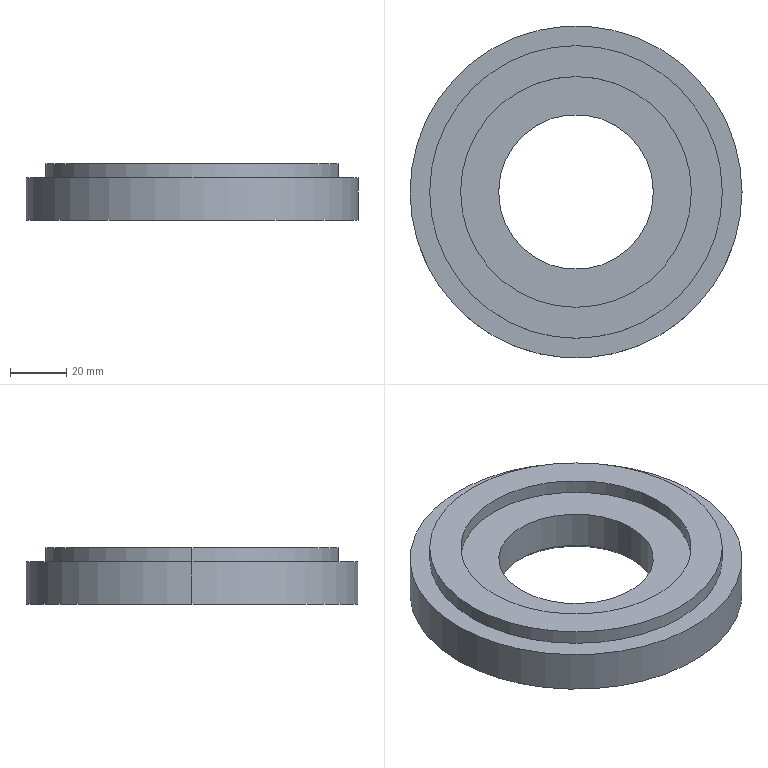Part | STEP file | Foot | 1 solid | 14 faces | box 118 x 118 x 20 mm | volume 144272 mm3 | cylinder 8 | plane 4 | cone 2 | commonest cylinder face diameters 55 x2 82 x2 104 x2 118 x2
STEP:
#1=CARTESIAN_POINT('',(0.,0.,0.));
#2=DIRECTION('',(0.,0.,1.));
#3=DIRECTION('',(1.,0.,0.));
#4=AXIS2_PLACEMENT_3D('',#1,#2,#3);
#5=CARTESIAN_POINT('',(-27.5,0.,1.5));
#6=VERTEX_POINT('',#5);
#7=CARTESIAN_POINT('',(-29.,0.,0.));
#8=VERTEX_POINT('',#7);
#9=CARTESIAN_POINT('',(-29.,0.,0.));
#10=DIRECTION('',(-0.7071,0.,-0.7071));
#11=VECTOR('',#10,1.);
#12=LINE('',#9,#11);
#13=CARTESIAN_POINT('',(0.,0.,0.));
#14=DIRECTION('',(0.,0.,-1.));
#15=DIRECTION('',(-1.,0.,0.));
#16=AXIS2_PLACEMENT_3D('',#13,#14,#15);
#17=CONICAL_SURFACE('',#16,29.,0.7854);
#18=CARTESIAN_POINT('',(6.283,0.));
#19=DIRECTION('',(0.,1.));
#20=VECTOR('',#19,1.);
#21=LINE('',#18,#20);
#22=(GEOMETRIC_REPRESENTATION_CONTEXT(2)PARAMETRIC_REPRESENTATION_CONTEXT()REPRESENTATION_CONTEXT('',''));
#23=DEFINITIONAL_REPRESENTATION('',(#21),#22);
#24=PCURVE('',#17,#23);
#25=CARTESIAN_POINT('',(0.,0.,0.));
#26=DIRECTION('',(0.,0.,-1.));
#27=DIRECTION('',(-1.,0.,0.));
#28=AXIS2_PLACEMENT_3D('',#25,#26,#27);
#29=CONICAL_SURFACE('',#28,29.,0.7854);
#30=CARTESIAN_POINT('',(0.,0.));
#31=DIRECTION('',(0.,1.));
#32=VECTOR('',#31,1.);
#33=LINE('',#30,#32);
#34=(GEOMETRIC_REPRESENTATION_CONTEXT(2)PARAMETRIC_REPRESENTATION_CONTEXT()REPRESENTATION_CONTEXT('',''));
#35=DEFINITIONAL_REPRESENTATION('',(#33),#34);
#36=PCURVE('',#29,#35);
#37=SURFACE_CURVE('',#12,(#24,#36),.PCURVE_S1.);
#38=EDGE_CURVE('',#6,#8,#37,.T.);
#39=ORIENTED_EDGE('',*,*,#38,.T.);
#40=CARTESIAN_POINT('',(29.,0.,0.));
#41=VERTEX_POINT('',#40);
#42=CARTESIAN_POINT('',(0.,0.,0.));
#43=DIRECTION('',(0.,0.,1.));
#44=DIRECTION('',(1.,0.,0.));
#45=AXIS2_PLACEMENT_3D('',#42,#43,#44);
#46=CIRCLE('',#45,29.);
#47=CARTESIAN_POINT('',(9.425,0.));
#48=DIRECTION('',(-1.,0.));
#49=VECTOR('',#48,1.);
#50=LINE('',#47,#49);
#51=(GEOMETRIC_REPRESENTATION_CONTEXT(2)PARAMETRIC_REPRESENTATION_CONTEXT()REPRESENTATION_CONTEXT('',''));
#52=DEFINITIONAL_REPRESENTATION('',(#50),#51);
#53=PCURVE('',#17,#52);
#54=CARTESIAN_POINT('',(0.,0.,0.));
#55=DIRECTION('',(0.,0.,1.));
#56=DIRECTION('',(1.,0.,0.));
#57=AXIS2_PLACEMENT_3D('',#54,#55,#56);
#58=PLANE('',#57);
#59=CARTESIAN_POINT('',(0.,0.));
#60=DIRECTION('',(1.,0.));
#61=AXIS2_PLACEMENT_2D('',#59,#60);
#62=CIRCLE('',#61,29.);
#63=(GEOMETRIC_REPRESENTATION_CONTEXT(2)PARAMETRIC_REPRESENTATION_CONTEXT()REPRESENTATION_CONTEXT('',''));
#64=DEFINITIONAL_REPRESENTATION('',(#62),#63);
#65=PCURVE('',#58,#64);
#66=SURFACE_CURVE('',#46,(#53,#65),.PCURVE_S1.);
#67=EDGE_CURVE('',#8,#41,#66,.T.);
#68=ORIENTED_EDGE('',*,*,#67,.T.);
#69=CARTESIAN_POINT('',(27.5,0.,1.5));
#70=VERTEX_POINT('',#69);
#71=CARTESIAN_POINT('',(29.,0.,0.));
#72=DIRECTION('',(0.7071,0.,-0.7071));
#73=VECTOR('',#72,1.);
#74=LINE('',#71,#73);
#75=CARTESIAN_POINT('',(3.142,0.));
#76=DIRECTION('',(0.,1.));
#77=VECTOR('',#76,1.);
#78=LINE('',#75,#77);
#79=(GEOMETRIC_REPRESENTATION_CONTEXT(2)PARAMETRIC_REPRESENTATION_CONTEXT()REPRESENTATION_CONTEXT('',''));
#80=DEFINITIONAL_REPRESENTATION('',(#78),#79);
#81=PCURVE('',#17,#80);
#82=CARTESIAN_POINT('',(3.142,0.));
#83=DIRECTION('',(0.,1.));
#84=VECTOR('',#83,1.);
#85=LINE('',#82,#84);
#86=(GEOMETRIC_REPRESENTATION_CONTEXT(2)PARAMETRIC_REPRESENTATION_CONTEXT()REPRESENTATION_CONTEXT('',''));
#87=DEFINITIONAL_REPRESENTATION('',(#85),#86);
#88=PCURVE('',#29,#87);
#89=SURFACE_CURVE('',#74,(#81,#88),.PCURVE_S1.);
#90=EDGE_CURVE('',#70,#41,#89,.T.);
#91=ORIENTED_EDGE('',*,*,#90,.F.);
#92=CARTESIAN_POINT('',(0.,0.,1.5));
#93=DIRECTION('',(0.,0.,-1.));
#94=DIRECTION('',(1.,0.,0.));
#95=AXIS2_PLACEMENT_3D('',#92,#93,#94);
#96=CIRCLE('',#95,27.5);
#97=CARTESIAN_POINT('',(3.142,-1.5));
#98=DIRECTION('',(1.,0.));
#99=VECTOR('',#98,1.);
#100=LINE('',#97,#99);
#101=(GEOMETRIC_REPRESENTATION_CONTEXT(2)PARAMETRIC_REPRESENTATION_CONTEXT()REPRESENTATION_CONTEXT('',''));
#102=DEFINITIONAL_REPRESENTATION('',(#100),#101);
#103=PCURVE('',#17,#102);
#104=CARTESIAN_POINT('',(0.,0.,15.));
#105=DIRECTION('',(0.,0.,-1.));
#106=DIRECTION('',(-1.,0.,0.));
#107=AXIS2_PLACEMENT_3D('',#104,#105,#106);
#108=CYLINDRICAL_SURFACE('',#107,27.5);
#109=CARTESIAN_POINT('',(3.142,13.5));
#110=DIRECTION('',(1.,0.));
#111=VECTOR('',#110,1.);
#112=LINE('',#109,#111);
#113=(GEOMETRIC_REPRESENTATION_CONTEXT(2)PARAMETRIC_REPRESENTATION_CONTEXT()REPRESENTATION_CONTEXT('',''));
#114=DEFINITIONAL_REPRESENTATION('',(#112),#113);
#115=PCURVE('',#108,#114);
#116=SURFACE_CURVE('',#96,(#103,#115),.PCURVE_S1.);
#117=EDGE_CURVE('',#70,#6,#116,.T.);
#118=ORIENTED_EDGE('',*,*,#117,.T.);
#119=EDGE_LOOP('',(#39,#68,#91,#118));
#120=FACE_BOUND('',#119,.F.);
#121=ADVANCED_FACE('',(#120),#17,.F.);
#122=CARTESIAN_POINT('',(-41.,0.,20.));
#123=VERTEX_POINT('',#122);
#124=CARTESIAN_POINT('',(-41.,0.,15.));
#125=VERTEX_POINT('',#124);
#126=CARTESIAN_POINT('',(-41.,0.,20.));
#127=DIRECTION('',(0.,0.,-1.));
#128=VECTOR('',#127,1.);
#129=LINE('',#126,#128);
#130=CARTESIAN_POINT('',(0.,0.,20.));
#131=DIRECTION('',(0.,0.,-1.));
#132=DIRECTION('',(-1.,0.,0.));
#133=AXIS2_PLACEMENT_3D('',#130,#131,#132);
#134=CYLINDRICAL_SURFACE('',#133,41.);
#135=CARTESIAN_POINT('',(6.283,0.));
#136=DIRECTION('',(0.,1.));
#137=VECTOR('',#136,1.);
#138=LINE('',#135,#137);
#139=(GEOMETRIC_REPRESENTATION_CONTEXT(2)PARAMETRIC_REPRESENTATION_CONTEXT()REPRESENTATION_CONTEXT('',''));
#140=DEFINITIONAL_REPRESENTATION('',(#138),#139);
#141=PCURVE('',#134,#140);
#142=CARTESIAN_POINT('',(0.,0.,20.));
#143=DIRECTION('',(0.,0.,-1.));
#144=DIRECTION('',(-1.,0.,0.));
#145=AXIS2_PLACEMENT_3D('',#142,#143,#144);
#146=CYLINDRICAL_SURFACE('',#145,41.);
#147=CARTESIAN_POINT('',(0.,0.));
#148=DIRECTION('',(0.,1.));
#149=VECTOR('',#148,1.);
#150=LINE('',#147,#149);
#151=(GEOMETRIC_REPRESENTATION_CONTEXT(2)PARAMETRIC_REPRESENTATION_CONTEXT()REPRESENTATION_CONTEXT('',''));
#152=DEFINITIONAL_REPRESENTATION('',(#150),#151);
#153=PCURVE('',#146,#152);
#154=SURFACE_CURVE('',#129,(#141,#153),.PCURVE_S1.);
#155=EDGE_CURVE('',#123,#125,#154,.T.);
#156=ORIENTED_EDGE('',*,*,#155,.T.);
#157=CARTESIAN_POINT('',(41.,0.,15.));
#158=VERTEX_POINT('',#157);
#159=CARTESIAN_POINT('',(0.,0.,15.));
#160=DIRECTION('',(0.,0.,-1.));
#161=DIRECTION('',(1.,0.,0.));
#162=AXIS2_PLACEMENT_3D('',#159,#160,#161);
#163=CIRCLE('',#162,41.);
#164=CARTESIAN_POINT('',(3.142,5.));
#165=DIRECTION('',(1.,0.));
#166=VECTOR('',#165,1.);
#167=LINE('',#164,#166);
#168=(GEOMETRIC_REPRESENTATION_CONTEXT(2)PARAMETRIC_REPRESENTATION_CONTEXT()REPRESENTATION_CONTEXT('',''));
#169=DEFINITIONAL_REPRESENTATION('',(#167),#168);
#170=PCURVE('',#134,#169);
#171=CARTESIAN_POINT('',(0.,0.,15.));
#172=DIRECTION('',(0.,0.,1.));
#173=DIRECTION('',(1.,0.,0.));
#174=AXIS2_PLACEMENT_3D('',#171,#172,#173);
#175=PLANE('',#174);
#176=CARTESIAN_POINT('',(41.,0.));
#177=CARTESIAN_POINT('',(41.,-71.014));
#178=CARTESIAN_POINT('',(-20.5,-35.507));
#179=CARTESIAN_POINT('',(-82.,0.));
#180=CARTESIAN_POINT('',(-20.5,35.507));
#181=CARTESIAN_POINT('',(41.,71.014));
#182=CARTESIAN_POINT('',(41.,0.));
#183=(BOUNDED_CURVE()B_SPLINE_CURVE(2,(#176,#177,#178,#179,#180,#181,#182),.UNSPECIFIED.,.T.,.F.)B_SPLINE_CURVE_WITH_KNOTS((1,2,2,2,2,1),(-2.094,0.,2.094,4.189,6.283,8.378),.UNSPECIFIED.)CURVE()GEOMETRIC_REPRESENTATION_ITEM()RATIONAL_B_SPLINE_CURVE((1.,0.5,1.,0.5,1.,0.5,1.))REPRESENTATION_ITEM(''));
#184=(GEOMETRIC_REPRESENTATION_CONTEXT(2)PARAMETRIC_REPRESENTATION_CONTEXT()REPRESENTATION_CONTEXT('',''));
#185=DEFINITIONAL_REPRESENTATION('',(#183),#184);
#186=PCURVE('',#175,#185);
#187=SURFACE_CURVE('',#163,(#170,#186),.PCURVE_S1.);
#188=EDGE_CURVE('',#158,#125,#187,.T.);
#189=ORIENTED_EDGE('',*,*,#188,.F.);
#190=CARTESIAN_POINT('',(41.,0.,20.));
#191=VERTEX_POINT('',#190);
#192=CARTESIAN_POINT('',(41.,0.,20.));
#193=DIRECTION('',(0.,0.,-1.));
#194=VECTOR('',#193,1.);
#195=LINE('',#192,#194);
#196=CARTESIAN_POINT('',(3.142,0.));
#197=DIRECTION('',(0.,1.));
#198=VECTOR('',#197,1.);
#199=LINE('',#196,#198);
#200=(GEOMETRIC_REPRESENTATION_CONTEXT(2)PARAMETRIC_REPRESENTATION_CONTEXT()REPRESENTATION_CONTEXT('',''));
#201=DEFINITIONAL_REPRESENTATION('',(#199),#200);
#202=PCURVE('',#134,#201);
#203=CARTESIAN_POINT('',(3.142,0.));
#204=DIRECTION('',(0.,1.));
#205=VECTOR('',#204,1.);
#206=LINE('',#203,#205);
#207=(GEOMETRIC_REPRESENTATION_CONTEXT(2)PARAMETRIC_REPRESENTATION_CONTEXT()REPRESENTATION_CONTEXT('',''));
#208=DEFINITIONAL_REPRESENTATION('',(#206),#207);
#209=PCURVE('',#146,#208);
#210=SURFACE_CURVE('',#195,(#202,#209),.PCURVE_S1.);
#211=EDGE_CURVE('',#191,#158,#210,.T.);
#212=ORIENTED_EDGE('',*,*,#211,.F.);
#213=CARTESIAN_POINT('',(0.,0.,20.));
#214=DIRECTION('',(0.,0.,1.));
#215=DIRECTION('',(1.,0.,0.));
#216=AXIS2_PLACEMENT_3D('',#213,#214,#215);
#217=CIRCLE('',#216,41.);
#218=CARTESIAN_POINT('',(9.425,0.));
#219=DIRECTION('',(-1.,0.));
#220=VECTOR('',#219,1.);
#221=LINE('',#218,#220);
#222=(GEOMETRIC_REPRESENTATION_CONTEXT(2)PARAMETRIC_REPRESENTATION_CONTEXT()REPRESENTATION_CONTEXT('',''));
#223=DEFINITIONAL_REPRESENTATION('',(#221),#222);
#224=PCURVE('',#134,#223);
#225=CARTESIAN_POINT('',(0.,0.,20.));
#226=DIRECTION('',(0.,0.,1.));
#227=DIRECTION('',(1.,0.,0.));
#228=AXIS2_PLACEMENT_3D('',#225,#226,#227);
#229=PLANE('',#228);
#230=CARTESIAN_POINT('',(0.,0.));
#231=DIRECTION('',(1.,0.));
#232=AXIS2_PLACEMENT_2D('',#230,#231);
#233=CIRCLE('',#232,41.);
#234=(GEOMETRIC_REPRESENTATION_CONTEXT(2)PARAMETRIC_REPRESENTATION_CONTEXT()REPRESENTATION_CONTEXT('',''));
#235=DEFINITIONAL_REPRESENTATION('',(#233),#234);
#236=PCURVE('',#229,#235);
#237=SURFACE_CURVE('',#217,(#224,#236),.PCURVE_S1.);
#238=EDGE_CURVE('',#123,#191,#237,.T.);
#239=ORIENTED_EDGE('',*,*,#238,.F.);
#240=EDGE_LOOP('',(#156,#189,#212,#239));
#241=FACE_BOUND('',#240,.F.);
#242=ADVANCED_FACE('',(#241),#134,.F.);
#243=CARTESIAN_POINT('',(52.,0.,20.));
#244=VERTEX_POINT('',#243);
#245=CARTESIAN_POINT('',(-52.,0.,20.));
#246=VERTEX_POINT('',#245);
#247=CARTESIAN_POINT('',(0.,0.,20.));
#248=DIRECTION('',(0.,0.,1.));
#249=DIRECTION('',(1.,0.,0.));
#250=AXIS2_PLACEMENT_3D('',#247,#248,#249);
#251=CIRCLE('',#250,52.);
#252=CARTESIAN_POINT('',(0.,0.,20.));
#253=DIRECTION('',(0.,0.,-1.));
#254=DIRECTION('',(-1.,0.,0.));
#255=AXIS2_PLACEMENT_3D('',#252,#253,#254);
#256=CYLINDRICAL_SURFACE('',#255,52.);
#257=CARTESIAN_POINT('',(3.142,0.));
#258=DIRECTION('',(-1.,0.));
#259=VECTOR('',#258,1.);
#260=LINE('',#257,#259);
#261=(GEOMETRIC_REPRESENTATION_CONTEXT(2)PARAMETRIC_REPRESENTATION_CONTEXT()REPRESENTATION_CONTEXT('',''));
#262=DEFINITIONAL_REPRESENTATION('',(#260),#261);
#263=PCURVE('',#256,#262);
#264=CARTESIAN_POINT('',(0.,0.));
#265=DIRECTION('',(1.,0.));
#266=AXIS2_PLACEMENT_2D('',#264,#265);
#267=CIRCLE('',#266,52.);
#268=(GEOMETRIC_REPRESENTATION_CONTEXT(2)PARAMETRIC_REPRESENTATION_CONTEXT()REPRESENTATION_CONTEXT('',''));
#269=DEFINITIONAL_REPRESENTATION('',(#267),#268);
#270=PCURVE('',#229,#269);
#271=SURFACE_CURVE('',#251,(#263,#270),.PCURVE_S1.);
#272=EDGE_CURVE('',#244,#246,#271,.T.);
#273=ORIENTED_EDGE('',*,*,#272,.F.);
#274=CARTESIAN_POINT('',(52.,0.,15.));
#275=VERTEX_POINT('',#274);
#276=CARTESIAN_POINT('',(52.,0.,20.));
#277=DIRECTION('',(0.,0.,-1.));
#278=VECTOR('',#277,1.);
#279=LINE('',#276,#278);
#280=CARTESIAN_POINT('',(3.142,0.));
#281=DIRECTION('',(0.,1.));
#282=VECTOR('',#281,1.);
#283=LINE('',#280,#282);
#284=(GEOMETRIC_REPRESENTATION_CONTEXT(2)PARAMETRIC_REPRESENTATION_CONTEXT()REPRESENTATION_CONTEXT('',''));
#285=DEFINITIONAL_REPRESENTATION('',(#283),#284);
#286=PCURVE('',#256,#285);
#287=CARTESIAN_POINT('',(0.,0.,20.));
#288=DIRECTION('',(0.,0.,-1.));
#289=DIRECTION('',(-1.,0.,0.));
#290=AXIS2_PLACEMENT_3D('',#287,#288,#289);
#291=CYLINDRICAL_SURFACE('',#290,52.);
#292=CARTESIAN_POINT('',(3.142,0.));
#293=DIRECTION('',(0.,1.));
#294=VECTOR('',#293,1.);
#295=LINE('',#292,#294);
#296=(GEOMETRIC_REPRESENTATION_CONTEXT(2)PARAMETRIC_REPRESENTATION_CONTEXT()REPRESENTATION_CONTEXT('',''));
#297=DEFINITIONAL_REPRESENTATION('',(#295),#296);
#298=PCURVE('',#291,#297);
#299=SURFACE_CURVE('',#279,(#286,#298),.PCURVE_S1.);
#300=EDGE_CURVE('',#244,#275,#299,.T.);
#301=ORIENTED_EDGE('',*,*,#300,.T.);
#302=CARTESIAN_POINT('',(-52.,0.,15.));
#303=VERTEX_POINT('',#302);
#304=CARTESIAN_POINT('',(0.,0.,15.));
#305=DIRECTION('',(0.,0.,1.));
#306=DIRECTION('',(1.,0.,0.));
#307=AXIS2_PLACEMENT_3D('',#304,#305,#306);
#308=CIRCLE('',#307,52.);
#309=CARTESIAN_POINT('',(3.142,5.));
#310=DIRECTION('',(-1.,0.));
#311=VECTOR('',#310,1.);
#312=LINE('',#309,#311);
#313=(GEOMETRIC_REPRESENTATION_CONTEXT(2)PARAMETRIC_REPRESENTATION_CONTEXT()REPRESENTATION_CONTEXT('',''));
#314=DEFINITIONAL_REPRESENTATION('',(#312),#313);
#315=PCURVE('',#256,#314);
#316=CARTESIAN_POINT('',(0.,0.,15.));
#317=DIRECTION('',(0.,0.,1.));
#318=DIRECTION('',(1.,0.,0.));
#319=AXIS2_PLACEMENT_3D('',#316,#317,#318);
#320=PLANE('',#319);
#321=CARTESIAN_POINT('',(0.,0.));
#322=DIRECTION('',(1.,0.));
#323=AXIS2_PLACEMENT_2D('',#321,#322);
#324=CIRCLE('',#323,52.);
#325=(GEOMETRIC_REPRESENTATION_CONTEXT(2)PARAMETRIC_REPRESENTATION_CONTEXT()REPRESENTATION_CONTEXT('',''));
#326=DEFINITIONAL_REPRESENTATION('',(#324),#325);
#327=PCURVE('',#320,#326);
#328=SURFACE_CURVE('',#308,(#315,#327),.PCURVE_S1.);
#329=EDGE_CURVE('',#275,#303,#328,.T.);
#330=ORIENTED_EDGE('',*,*,#329,.T.);
#331=CARTESIAN_POINT('',(-52.,0.,20.));
#332=DIRECTION('',(0.,0.,-1.));
#333=VECTOR('',#332,1.);
#334=LINE('',#331,#333);
#335=CARTESIAN_POINT('',(0.,0.));
#336=DIRECTION('',(0.,1.));
#337=VECTOR('',#336,1.);
#338=LINE('',#335,#337);
#339=(GEOMETRIC_REPRESENTATION_CONTEXT(2)PARAMETRIC_REPRESENTATION_CONTEXT()REPRESENTATION_CONTEXT('',''));
#340=DEFINITIONAL_REPRESENTATION('',(#338),#339);
#341=PCURVE('',#256,#340);
#342=CARTESIAN_POINT('',(6.283,0.));
#343=DIRECTION('',(0.,1.));
#344=VECTOR('',#343,1.);
#345=LINE('',#342,#344);
#346=(GEOMETRIC_REPRESENTATION_CONTEXT(2)PARAMETRIC_REPRESENTATION_CONTEXT()REPRESENTATION_CONTEXT('',''));
#347=DEFINITIONAL_REPRESENTATION('',(#345),#346);
#348=PCURVE('',#291,#347);
#349=SURFACE_CURVE('',#334,(#341,#348),.PCURVE_S1.);
#350=EDGE_CURVE('',#246,#303,#349,.T.);
#351=ORIENTED_EDGE('',*,*,#350,.F.);
#352=EDGE_LOOP('',(#273,#301,#330,#351));
#353=FACE_BOUND('',#352,.T.);
#354=ADVANCED_FACE('',(#353),#256,.T.);
#355=CARTESIAN_POINT('',(-27.5,0.,15.));
#356=VERTEX_POINT('',#355);
#357=CARTESIAN_POINT('',(-27.5,0.,15.));
#358=DIRECTION('',(0.,0.,-1.));
#359=VECTOR('',#358,1.);
#360=LINE('',#357,#359);
#361=CARTESIAN_POINT('',(6.283,0.));
#362=DIRECTION('',(0.,1.));
#363=VECTOR('',#362,1.);
#364=LINE('',#361,#363);
#365=(GEOMETRIC_REPRESENTATION_CONTEXT(2)PARAMETRIC_REPRESENTATION_CONTEXT()REPRESENTATION_CONTEXT('',''));
#366=DEFINITIONAL_REPRESENTATION('',(#364),#365);
#367=PCURVE('',#108,#366);
#368=CARTESIAN_POINT('',(0.,0.,15.));
#369=DIRECTION('',(0.,0.,-1.));
#370=DIRECTION('',(-1.,0.,0.));
#371=AXIS2_PLACEMENT_3D('',#368,#369,#370);
#372=CYLINDRICAL_SURFACE('',#371,27.5);
#373=CARTESIAN_POINT('',(0.,0.));
#374=DIRECTION('',(0.,1.));
#375=VECTOR('',#374,1.);
#376=LINE('',#373,#375);
#377=(GEOMETRIC_REPRESENTATION_CONTEXT(2)PARAMETRIC_REPRESENTATION_CONTEXT()REPRESENTATION_CONTEXT('',''));
#378=DEFINITIONAL_REPRESENTATION('',(#376),#377);
#379=PCURVE('',#372,#378);
#380=SURFACE_CURVE('',#360,(#367,#379),.PCURVE_S1.);
#381=EDGE_CURVE('',#356,#6,#380,.T.);
#382=ORIENTED_EDGE('',*,*,#381,.T.);
#383=ORIENTED_EDGE('',*,*,#117,.F.);
#384=CARTESIAN_POINT('',(27.5,0.,15.));
#385=VERTEX_POINT('',#384);
#386=CARTESIAN_POINT('',(27.5,0.,15.));
#387=DIRECTION('',(0.,0.,-1.));
#388=VECTOR('',#387,1.);
#389=LINE('',#386,#388);
#390=CARTESIAN_POINT('',(3.142,0.));
#391=DIRECTION('',(0.,1.));
#392=VECTOR('',#391,1.);
#393=LINE('',#390,#392);
#394=(GEOMETRIC_REPRESENTATION_CONTEXT(2)PARAMETRIC_REPRESENTATION_CONTEXT()REPRESENTATION_CONTEXT('',''));
#395=DEFINITIONAL_REPRESENTATION('',(#393),#394);
#396=PCURVE('',#108,#395);
#397=CARTESIAN_POINT('',(3.142,0.));
#398=DIRECTION('',(0.,1.));
#399=VECTOR('',#398,1.);
#400=LINE('',#397,#399);
#401=(GEOMETRIC_REPRESENTATION_CONTEXT(2)PARAMETRIC_REPRESENTATION_CONTEXT()REPRESENTATION_CONTEXT('',''));
#402=DEFINITIONAL_REPRESENTATION('',(#400),#401);
#403=PCURVE('',#372,#402);
#404=SURFACE_CURVE('',#389,(#396,#403),.PCURVE_S1.);
#405=EDGE_CURVE('',#385,#70,#404,.T.);
#406=ORIENTED_EDGE('',*,*,#405,.F.);
#407=CARTESIAN_POINT('',(0.,0.,15.));
#408=DIRECTION('',(0.,0.,1.));
#409=DIRECTION('',(1.,0.,0.));
#410=AXIS2_PLACEMENT_3D('',#407,#408,#409);
#411=CIRCLE('',#410,27.5);
#412=CARTESIAN_POINT('',(9.425,0.));
#413=DIRECTION('',(-1.,0.));
#414=VECTOR('',#413,1.);
#415=LINE('',#412,#414);
#416=(GEOMETRIC_REPRESENTATION_CONTEXT(2)PARAMETRIC_REPRESENTATION_CONTEXT()REPRESENTATION_CONTEXT('',''));
#417=DEFINITIONAL_REPRESENTATION('',(#415),#416);
#418=PCURVE('',#108,#417);
#419=CARTESIAN_POINT('',(0.,0.));
#420=DIRECTION('',(1.,0.));
#421=AXIS2_PLACEMENT_2D('',#419,#420);
#422=CIRCLE('',#421,27.5);
#423=(GEOMETRIC_REPRESENTATION_CONTEXT(2)PARAMETRIC_REPRESENTATION_CONTEXT()REPRESENTATION_CONTEXT('',''));
#424=DEFINITIONAL_REPRESENTATION('',(#422),#423);
#425=PCURVE('',#175,#424);
#426=SURFACE_CURVE('',#411,(#418,#425),.PCURVE_S1.);
#427=EDGE_CURVE('',#356,#385,#426,.T.);
#428=ORIENTED_EDGE('',*,*,#427,.F.);
#429=EDGE_LOOP('',(#382,#383,#406,#428));
#430=FACE_BOUND('',#429,.F.);
#431=ADVANCED_FACE('',(#430),#108,.F.);
#432=CARTESIAN_POINT('',(59.,0.,15.));
#433=VERTEX_POINT('',#432);
#434=CARTESIAN_POINT('',(-59.,0.,15.));
#435=VERTEX_POINT('',#434);
#436=CARTESIAN_POINT('',(0.,0.,15.));
#437=DIRECTION('',(0.,0.,1.));
#438=DIRECTION('',(1.,0.,0.));
#439=AXIS2_PLACEMENT_3D('',#436,#437,#438);
#440=CIRCLE('',#439,59.);
#441=CARTESIAN_POINT('',(0.,0.,15.));
#442=DIRECTION('',(0.,0.,-1.));
#443=DIRECTION('',(-1.,0.,0.));
#444=AXIS2_PLACEMENT_3D('',#441,#442,#443);
#445=CYLINDRICAL_SURFACE('',#444,59.);
#446=CARTESIAN_POINT('',(3.142,0.));
#447=DIRECTION('',(-1.,0.));
#448=VECTOR('',#447,1.);
#449=LINE('',#446,#448);
#450=(GEOMETRIC_REPRESENTATION_CONTEXT(2)PARAMETRIC_REPRESENTATION_CONTEXT()REPRESENTATION_CONTEXT('',''));
#451=DEFINITIONAL_REPRESENTATION('',(#449),#450);
#452=PCURVE('',#445,#451);
#453=CARTESIAN_POINT('',(0.,0.));
#454=DIRECTION('',(1.,0.));
#455=AXIS2_PLACEMENT_2D('',#453,#454);
#456=CIRCLE('',#455,59.);
#457=(GEOMETRIC_REPRESENTATION_CONTEXT(2)PARAMETRIC_REPRESENTATION_CONTEXT()REPRESENTATION_CONTEXT('',''));
#458=DEFINITIONAL_REPRESENTATION('',(#456),#457);
#459=PCURVE('',#320,#458);
#460=SURFACE_CURVE('',#440,(#452,#459),.PCURVE_S1.);
#461=EDGE_CURVE('',#433,#435,#460,.T.);
#462=ORIENTED_EDGE('',*,*,#461,.F.);
#463=CARTESIAN_POINT('',(59.,0.,0.));
#464=VERTEX_POINT('',#463);
#465=CARTESIAN_POINT('',(59.,0.,15.));
#466=DIRECTION('',(0.,0.,-1.));
#467=VECTOR('',#466,1.);
#468=LINE('',#465,#467);
#469=CARTESIAN_POINT('',(3.142,0.));
#470=DIRECTION('',(0.,1.));
#471=VECTOR('',#470,1.);
#472=LINE('',#469,#471);
#473=(GEOMETRIC_REPRESENTATION_CONTEXT(2)PARAMETRIC_REPRESENTATION_CONTEXT()REPRESENTATION_CONTEXT('',''));
#474=DEFINITIONAL_REPRESENTATION('',(#472),#473);
#475=PCURVE('',#445,#474);
#476=CARTESIAN_POINT('',(0.,0.,15.));
#477=DIRECTION('',(0.,0.,-1.));
#478=DIRECTION('',(-1.,0.,0.));
#479=AXIS2_PLACEMENT_3D('',#476,#477,#478);
#480=CYLINDRICAL_SURFACE('',#479,59.);
#481=CARTESIAN_POINT('',(3.142,0.));
#482=DIRECTION('',(0.,1.));
#483=VECTOR('',#482,1.);
#484=LINE('',#481,#483);
#485=(GEOMETRIC_REPRESENTATION_CONTEXT(2)PARAMETRIC_REPRESENTATION_CONTEXT()REPRESENTATION_CONTEXT('',''));
#486=DEFINITIONAL_REPRESENTATION('',(#484),#485);
#487=PCURVE('',#480,#486);
#488=SURFACE_CURVE('',#468,(#475,#487),.PCURVE_S1.);
#489=EDGE_CURVE('',#433,#464,#488,.T.);
#490=ORIENTED_EDGE('',*,*,#489,.T.);
#491=CARTESIAN_POINT('',(-59.,0.,0.));
#492=VERTEX_POINT('',#491);
#493=CARTESIAN_POINT('',(0.,0.,0.));
#494=DIRECTION('',(0.,0.,1.));
#495=DIRECTION('',(1.,0.,0.));
#496=AXIS2_PLACEMENT_3D('',#493,#494,#495);
#497=CIRCLE('',#496,59.);
#498=CARTESIAN_POINT('',(3.142,15.));
#499=DIRECTION('',(-1.,0.));
#500=VECTOR('',#499,1.);
#501=LINE('',#498,#500);
#502=(GEOMETRIC_REPRESENTATION_CONTEXT(2)PARAMETRIC_REPRESENTATION_CONTEXT()REPRESENTATION_CONTEXT('',''));
#503=DEFINITIONAL_REPRESENTATION('',(#501),#502);
#504=PCURVE('',#445,#503);
#505=CARTESIAN_POINT('',(0.,0.));
#506=DIRECTION('',(1.,0.));
#507=AXIS2_PLACEMENT_2D('',#505,#506);
#508=CIRCLE('',#507,59.);
#509=(GEOMETRIC_REPRESENTATION_CONTEXT(2)PARAMETRIC_REPRESENTATION_CONTEXT()REPRESENTATION_CONTEXT('',''));
#510=DEFINITIONAL_REPRESENTATION('',(#508),#509);
#511=PCURVE('',#58,#510);
#512=SURFACE_CURVE('',#497,(#504,#511),.PCURVE_S1.);
#513=EDGE_CURVE('',#464,#492,#512,.T.);
#514=ORIENTED_EDGE('',*,*,#513,.T.);
#515=CARTESIAN_POINT('',(-59.,0.,15.));
#516=DIRECTION('',(0.,0.,-1.));
#517=VECTOR('',#516,1.);
#518=LINE('',#515,#517);
#519=CARTESIAN_POINT('',(0.,0.));
#520=DIRECTION('',(0.,1.));
#521=VECTOR('',#520,1.);
#522=LINE('',#519,#521);
#523=(GEOMETRIC_REPRESENTATION_CONTEXT(2)PARAMETRIC_REPRESENTATION_CONTEXT()REPRESENTATION_CONTEXT('',''));
#524=DEFINITIONAL_REPRESENTATION('',(#522),#523);
#525=PCURVE('',#445,#524);
#526=CARTESIAN_POINT('',(6.283,0.));
#527=DIRECTION('',(0.,1.));
#528=VECTOR('',#527,1.);
#529=LINE('',#526,#528);
#530=(GEOMETRIC_REPRESENTATION_CONTEXT(2)PARAMETRIC_REPRESENTATION_CONTEXT()REPRESENTATION_CONTEXT('',''));
#531=DEFINITIONAL_REPRESENTATION('',(#529),#530);
#532=PCURVE('',#480,#531);
#533=SURFACE_CURVE('',#518,(#525,#532),.PCURVE_S1.);
#534=EDGE_CURVE('',#435,#492,#533,.T.);
#535=ORIENTED_EDGE('',*,*,#534,.F.);
#536=EDGE_LOOP('',(#462,#490,#514,#535));
#537=FACE_BOUND('',#536,.T.);
#538=ADVANCED_FACE('',(#537),#445,.T.);
#539=CARTESIAN_POINT('',(0.,0.,15.));
#540=DIRECTION('',(0.,0.,1.));
#541=DIRECTION('',(1.,0.,0.));
#542=AXIS2_PLACEMENT_3D('',#539,#540,#541);
#543=CIRCLE('',#542,59.);
#544=CARTESIAN_POINT('',(0.,0.));
#545=DIRECTION('',(1.,0.));
#546=AXIS2_PLACEMENT_2D('',#544,#545);
#547=CIRCLE('',#546,59.);
#548=(GEOMETRIC_REPRESENTATION_CONTEXT(2)PARAMETRIC_REPRESENTATION_CONTEXT()REPRESENTATION_CONTEXT('',''));
#549=DEFINITIONAL_REPRESENTATION('',(#547),#548);
#550=PCURVE('',#320,#549);
#551=CARTESIAN_POINT('',(9.425,0.));
#552=DIRECTION('',(-1.,0.));
#553=VECTOR('',#552,1.);
#554=LINE('',#551,#553);
#555=(GEOMETRIC_REPRESENTATION_CONTEXT(2)PARAMETRIC_REPRESENTATION_CONTEXT()REPRESENTATION_CONTEXT('',''));
#556=DEFINITIONAL_REPRESENTATION('',(#554),#555);
#557=PCURVE('',#480,#556);
#558=SURFACE_CURVE('',#543,(#550,#557),.PCURVE_S1.);
#559=EDGE_CURVE('',#435,#433,#558,.T.);
#560=ORIENTED_EDGE('',*,*,#559,.T.);
#561=ORIENTED_EDGE('',*,*,#461,.T.);
#562=EDGE_LOOP('',(#560,#561));
#563=FACE_BOUND('',#562,.T.);
#564=CARTESIAN_POINT('',(0.,0.,15.));
#565=DIRECTION('',(0.,0.,1.));
#566=DIRECTION('',(1.,0.,0.));
#567=AXIS2_PLACEMENT_3D('',#564,#565,#566);
#568=CIRCLE('',#567,52.);
#569=CARTESIAN_POINT('',(0.,0.));
#570=DIRECTION('',(1.,0.));
#571=AXIS2_PLACEMENT_2D('',#569,#570);
#572=CIRCLE('',#571,52.);
#573=(GEOMETRIC_REPRESENTATION_CONTEXT(2)PARAMETRIC_REPRESENTATION_CONTEXT()REPRESENTATION_CONTEXT('',''));
#574=DEFINITIONAL_REPRESENTATION('',(#572),#573);
#575=PCURVE('',#320,#574);
#576=CARTESIAN_POINT('',(9.425,5.));
#577=DIRECTION('',(-1.,0.));
#578=VECTOR('',#577,1.);
#579=LINE('',#576,#578);
#580=(GEOMETRIC_REPRESENTATION_CONTEXT(2)PARAMETRIC_REPRESENTATION_CONTEXT()REPRESENTATION_CONTEXT('',''));
#581=DEFINITIONAL_REPRESENTATION('',(#579),#580);
#582=PCURVE('',#291,#581);
#583=SURFACE_CURVE('',#568,(#575,#582),.PCURVE_S1.);
#584=EDGE_CURVE('',#303,#275,#583,.T.);
#585=ORIENTED_EDGE('',*,*,#584,.F.);
#586=ORIENTED_EDGE('',*,*,#329,.F.);
#587=EDGE_LOOP('',(#585,#586));
#588=FACE_BOUND('',#587,.T.);
#589=ADVANCED_FACE('',(#563,#588),#320,.T.);
#590=CARTESIAN_POINT('',(0.,0.,15.));
#591=DIRECTION('',(0.,0.,-1.));
#592=DIRECTION('',(1.,0.,0.));
#593=AXIS2_PLACEMENT_3D('',#590,#591,#592);
#594=CIRCLE('',#593,41.);
#595=CARTESIAN_POINT('',(41.,0.));
#596=CARTESIAN_POINT('',(41.,-71.014));
#597=CARTESIAN_POINT('',(-20.5,-35.507));
#598=CARTESIAN_POINT('',(-82.,0.));
#599=CARTESIAN_POINT('',(-20.5,35.507));
#600=CARTESIAN_POINT('',(41.,71.014));
#601=CARTESIAN_POINT('',(41.,0.));
#602=(BOUNDED_CURVE()B_SPLINE_CURVE(2,(#595,#596,#597,#598,#599,#600,#601),.UNSPECIFIED.,.T.,.F.)B_SPLINE_CURVE_WITH_KNOTS((1,2,2,2,2,1),(-2.094,0.,2.094,4.189,6.283,8.378),.UNSPECIFIED.)CURVE()GEOMETRIC_REPRESENTATION_ITEM()RATIONAL_B_SPLINE_CURVE((1.,0.5,1.,0.5,1.,0.5,1.))REPRESENTATION_ITEM(''));
#603=(GEOMETRIC_REPRESENTATION_CONTEXT(2)PARAMETRIC_REPRESENTATION_CONTEXT()REPRESENTATION_CONTEXT('',''));
#604=DEFINITIONAL_REPRESENTATION('',(#602),#603);
#605=PCURVE('',#175,#604);
#606=CARTESIAN_POINT('',(-3.142,5.));
#607=DIRECTION('',(1.,0.));
#608=VECTOR('',#607,1.);
#609=LINE('',#606,#608);
#610=(GEOMETRIC_REPRESENTATION_CONTEXT(2)PARAMETRIC_REPRESENTATION_CONTEXT()REPRESENTATION_CONTEXT('',''));
#611=DEFINITIONAL_REPRESENTATION('',(#609),#610);
#612=PCURVE('',#146,#611);
#613=SURFACE_CURVE('',#594,(#605,#612),.PCURVE_S1.);
#614=EDGE_CURVE('',#125,#158,#613,.T.);
#615=ORIENTED_EDGE('',*,*,#614,.F.);
#616=ORIENTED_EDGE('',*,*,#188,.F.);
#617=EDGE_LOOP('',(#615,#616));
#618=FACE_BOUND('',#617,.T.);
#619=ORIENTED_EDGE('',*,*,#427,.F.);
#620=CARTESIAN_POINT('',(0.,0.,15.));
#621=DIRECTION('',(0.,0.,1.));
#622=DIRECTION('',(1.,0.,0.));
#623=AXIS2_PLACEMENT_3D('',#620,#621,#622);
#624=CIRCLE('',#623,27.5);
#625=CARTESIAN_POINT('',(0.,0.));
#626=DIRECTION('',(1.,0.));
#627=AXIS2_PLACEMENT_2D('',#625,#626);
#628=CIRCLE('',#627,27.5);
#629=(GEOMETRIC_REPRESENTATION_CONTEXT(2)PARAMETRIC_REPRESENTATION_CONTEXT()REPRESENTATION_CONTEXT('',''));
#630=DEFINITIONAL_REPRESENTATION('',(#628),#629);
#631=PCURVE('',#175,#630);
#632=CARTESIAN_POINT('',(3.142,0.));
#633=DIRECTION('',(-1.,0.));
#634=VECTOR('',#633,1.);
#635=LINE('',#632,#634);
#636=(GEOMETRIC_REPRESENTATION_CONTEXT(2)PARAMETRIC_REPRESENTATION_CONTEXT()REPRESENTATION_CONTEXT('',''));
#637=DEFINITIONAL_REPRESENTATION('',(#635),#636);
#638=PCURVE('',#372,#637);
#639=SURFACE_CURVE('',#624,(#631,#638),.PCURVE_S1.);
#640=EDGE_CURVE('',#385,#356,#639,.T.);
#641=ORIENTED_EDGE('',*,*,#640,.F.);
#642=EDGE_LOOP('',(#619,#641));
#643=FACE_BOUND('',#642,.T.);
#644=ADVANCED_FACE('',(#618,#643),#175,.T.);
#645=ORIENTED_EDGE('',*,*,#67,.T.);
#646=CARTESIAN_POINT('',(0.,0.,0.));
#647=DIRECTION('',(0.,0.,1.));
#648=DIRECTION('',(1.,0.,0.));
#649=AXIS2_PLACEMENT_3D('',#646,#647,#648);
#650=CIRCLE('',#649,29.);
#651=CARTESIAN_POINT('',(0.,0.));
#652=DIRECTION('',(1.,0.));
#653=AXIS2_PLACEMENT_2D('',#651,#652);
#654=CIRCLE('',#653,29.);
#655=(GEOMETRIC_REPRESENTATION_CONTEXT(2)PARAMETRIC_REPRESENTATION_CONTEXT()REPRESENTATION_CONTEXT('',''));
#656=DEFINITIONAL_REPRESENTATION('',(#654),#655);
#657=PCURVE('',#58,#656);
#658=CARTESIAN_POINT('',(3.142,0.));
#659=DIRECTION('',(-1.,0.));
#660=VECTOR('',#659,1.);
#661=LINE('',#658,#660);
#662=(GEOMETRIC_REPRESENTATION_CONTEXT(2)PARAMETRIC_REPRESENTATION_CONTEXT()REPRESENTATION_CONTEXT('',''));
#663=DEFINITIONAL_REPRESENTATION('',(#661),#662);
#664=PCURVE('',#29,#663);
#665=SURFACE_CURVE('',#650,(#657,#664),.PCURVE_S1.);
#666=EDGE_CURVE('',#41,#8,#665,.T.);
#667=ORIENTED_EDGE('',*,*,#666,.T.);
#668=EDGE_LOOP('',(#645,#667));
#669=FACE_BOUND('',#668,.T.);
#670=CARTESIAN_POINT('',(0.,0.,0.));
#671=DIRECTION('',(0.,0.,1.));
#672=DIRECTION('',(1.,0.,0.));
#673=AXIS2_PLACEMENT_3D('',#670,#671,#672);
#674=CIRCLE('',#673,59.);
#675=CARTESIAN_POINT('',(0.,0.));
#676=DIRECTION('',(1.,0.));
#677=AXIS2_PLACEMENT_2D('',#675,#676);
#678=CIRCLE('',#677,59.);
#679=(GEOMETRIC_REPRESENTATION_CONTEXT(2)PARAMETRIC_REPRESENTATION_CONTEXT()REPRESENTATION_CONTEXT('',''));
#680=DEFINITIONAL_REPRESENTATION('',(#678),#679);
#681=PCURVE('',#58,#680);
#682=CARTESIAN_POINT('',(9.425,15.));
#683=DIRECTION('',(-1.,0.));
#684=VECTOR('',#683,1.);
#685=LINE('',#682,#684);
#686=(GEOMETRIC_REPRESENTATION_CONTEXT(2)PARAMETRIC_REPRESENTATION_CONTEXT()REPRESENTATION_CONTEXT('',''));
#687=DEFINITIONAL_REPRESENTATION('',(#685),#686);
#688=PCURVE('',#480,#687);
#689=SURFACE_CURVE('',#674,(#681,#688),.PCURVE_S1.);
#690=EDGE_CURVE('',#492,#464,#689,.T.);
#691=ORIENTED_EDGE('',*,*,#690,.F.);
#692=ORIENTED_EDGE('',*,*,#513,.F.);
#693=EDGE_LOOP('',(#691,#692));
#694=FACE_BOUND('',#693,.T.);
#695=ADVANCED_FACE('',(#669,#694),#58,.F.);
#696=ORIENTED_EDGE('',*,*,#489,.F.);
#697=ORIENTED_EDGE('',*,*,#559,.F.);
#698=ORIENTED_EDGE('',*,*,#534,.T.);
#699=ORIENTED_EDGE('',*,*,#690,.T.);
#700=EDGE_LOOP('',(#696,#697,#698,#699));
#701=FACE_BOUND('',#700,.T.);
#702=ADVANCED_FACE('',(#701),#480,.T.);
#703=CARTESIAN_POINT('',(0.,0.,1.5));
#704=DIRECTION('',(0.,0.,-1.));
#705=DIRECTION('',(1.,0.,0.));
#706=AXIS2_PLACEMENT_3D('',#703,#704,#705);
#707=CIRCLE('',#706,27.5);
#708=CARTESIAN_POINT('',(-3.142,13.5));
#709=DIRECTION('',(1.,0.));
#710=VECTOR('',#709,1.);
#711=LINE('',#708,#710);
#712=(GEOMETRIC_REPRESENTATION_CONTEXT(2)PARAMETRIC_REPRESENTATION_CONTEXT()REPRESENTATION_CONTEXT('',''));
#713=DEFINITIONAL_REPRESENTATION('',(#711),#712);
#714=PCURVE('',#372,#713);
#715=CARTESIAN_POINT('',(-3.142,-1.5));
#716=DIRECTION('',(1.,0.));
#717=VECTOR('',#716,1.);
#718=LINE('',#715,#717);
#719=(GEOMETRIC_REPRESENTATION_CONTEXT(2)PARAMETRIC_REPRESENTATION_CONTEXT()REPRESENTATION_CONTEXT('',''));
#720=DEFINITIONAL_REPRESENTATION('',(#718),#719);
#721=PCURVE('',#29,#720);
#722=SURFACE_CURVE('',#707,(#714,#721),.PCURVE_S1.);
#723=EDGE_CURVE('',#6,#70,#722,.T.);
#724=ORIENTED_EDGE('',*,*,#723,.F.);
#725=ORIENTED_EDGE('',*,*,#381,.F.);
#726=ORIENTED_EDGE('',*,*,#640,.F.);
#727=ORIENTED_EDGE('',*,*,#405,.T.);
#728=EDGE_LOOP('',(#724,#725,#726,#727));
#729=FACE_BOUND('',#728,.F.);
#730=ADVANCED_FACE('',(#729),#372,.F.);
#731=CARTESIAN_POINT('',(0.,0.,20.));
#732=DIRECTION('',(0.,0.,1.));
#733=DIRECTION('',(1.,0.,0.));
#734=AXIS2_PLACEMENT_3D('',#731,#732,#733);
#735=CIRCLE('',#734,52.);
#736=CARTESIAN_POINT('',(0.,0.));
#737=DIRECTION('',(1.,0.));
#738=AXIS2_PLACEMENT_2D('',#736,#737);
#739=CIRCLE('',#738,52.);
#740=(GEOMETRIC_REPRESENTATION_CONTEXT(2)PARAMETRIC_REPRESENTATION_CONTEXT()REPRESENTATION_CONTEXT('',''));
#741=DEFINITIONAL_REPRESENTATION('',(#739),#740);
#742=PCURVE('',#229,#741);
#743=CARTESIAN_POINT('',(9.425,0.));
#744=DIRECTION('',(-1.,0.));
#745=VECTOR('',#744,1.);
#746=LINE('',#743,#745);
#747=(GEOMETRIC_REPRESENTATION_CONTEXT(2)PARAMETRIC_REPRESENTATION_CONTEXT()REPRESENTATION_CONTEXT('',''));
#748=DEFINITIONAL_REPRESENTATION('',(#746),#747);
#749=PCURVE('',#291,#748);
#750=SURFACE_CURVE('',#735,(#742,#749),.PCURVE_S1.);
#751=EDGE_CURVE('',#246,#244,#750,.T.);
#752=ORIENTED_EDGE('',*,*,#751,.T.);
#753=ORIENTED_EDGE('',*,*,#272,.T.);
#754=EDGE_LOOP('',(#752,#753));
#755=FACE_BOUND('',#754,.T.);
#756=ORIENTED_EDGE('',*,*,#238,.F.);
#757=CARTESIAN_POINT('',(0.,0.,20.));
#758=DIRECTION('',(0.,0.,1.));
#759=DIRECTION('',(1.,0.,0.));
#760=AXIS2_PLACEMENT_3D('',#757,#758,#759);
#761=CIRCLE('',#760,41.);
#762=CARTESIAN_POINT('',(0.,0.));
#763=DIRECTION('',(1.,0.));
#764=AXIS2_PLACEMENT_2D('',#762,#763);
#765=CIRCLE('',#764,41.);
#766=(GEOMETRIC_REPRESENTATION_CONTEXT(2)PARAMETRIC_REPRESENTATION_CONTEXT()REPRESENTATION_CONTEXT('',''));
#767=DEFINITIONAL_REPRESENTATION('',(#765),#766);
#768=PCURVE('',#229,#767);
#769=CARTESIAN_POINT('',(3.142,0.));
#770=DIRECTION('',(-1.,0.));
#771=VECTOR('',#770,1.);
#772=LINE('',#769,#771);
#773=(GEOMETRIC_REPRESENTATION_CONTEXT(2)PARAMETRIC_REPRESENTATION_CONTEXT()REPRESENTATION_CONTEXT('',''));
#774=DEFINITIONAL_REPRESENTATION('',(#772),#773);
#775=PCURVE('',#146,#774);
#776=SURFACE_CURVE('',#761,(#768,#775),.PCURVE_S1.);
#777=EDGE_CURVE('',#191,#123,#776,.T.);
#778=ORIENTED_EDGE('',*,*,#777,.F.);
#779=EDGE_LOOP('',(#756,#778));
#780=FACE_BOUND('',#779,.T.);
#781=ADVANCED_FACE('',(#755,#780),#229,.T.);
#782=ORIENTED_EDGE('',*,*,#300,.F.);
#783=ORIENTED_EDGE('',*,*,#751,.F.);
#784=ORIENTED_EDGE('',*,*,#350,.T.);
#785=ORIENTED_EDGE('',*,*,#584,.T.);
#786=EDGE_LOOP('',(#782,#783,#784,#785));
#787=FACE_BOUND('',#786,.T.);
#788=ADVANCED_FACE('',(#787),#291,.T.);
#789=ORIENTED_EDGE('',*,*,#614,.F.);
#790=ORIENTED_EDGE('',*,*,#155,.F.);
#791=ORIENTED_EDGE('',*,*,#777,.F.);
#792=ORIENTED_EDGE('',*,*,#211,.T.);
#793=EDGE_LOOP('',(#789,#790,#791,#792));
#794=FACE_BOUND('',#793,.F.);
#795=ADVANCED_FACE('',(#794),#146,.F.);
#796=ORIENTED_EDGE('',*,*,#666,.T.);
#797=ORIENTED_EDGE('',*,*,#38,.F.);
#798=ORIENTED_EDGE('',*,*,#723,.T.);
#799=ORIENTED_EDGE('',*,*,#90,.T.);
#800=EDGE_LOOP('',(#796,#797,#798,#799));
#801=FACE_BOUND('',#800,.F.);
#802=ADVANCED_FACE('',(#801),#29,.F.);
#803=CLOSED_SHELL('',(#121,#242,#354,#431,#538,#589,#644,#695,#702,#730,#781,#788,#795,#802));
#804=MANIFOLD_SOLID_BREP('',#803);
#805=(LENGTH_UNIT()NAMED_UNIT(*)SI_UNIT(.MILLI.,.METRE.));
#806=UNCERTAINTY_MEASURE_WITH_UNIT(LENGTH_MEASURE(0.0000001),#805,'','');
#807=(NAMED_UNIT(*)PLANE_ANGLE_UNIT()SI_UNIT($,.RADIAN.));
#808=(NAMED_UNIT(*)SI_UNIT($,.STERADIAN.)SOLID_ANGLE_UNIT());
#809=(GEOMETRIC_REPRESENTATION_CONTEXT(3)GLOBAL_UNCERTAINTY_ASSIGNED_CONTEXT((#806))GLOBAL_UNIT_ASSIGNED_CONTEXT((#805,#807,#808))REPRESENTATION_CONTEXT('',''));
#810=ADVANCED_BREP_SHAPE_REPRESENTATION('',(#4,#804),#809);